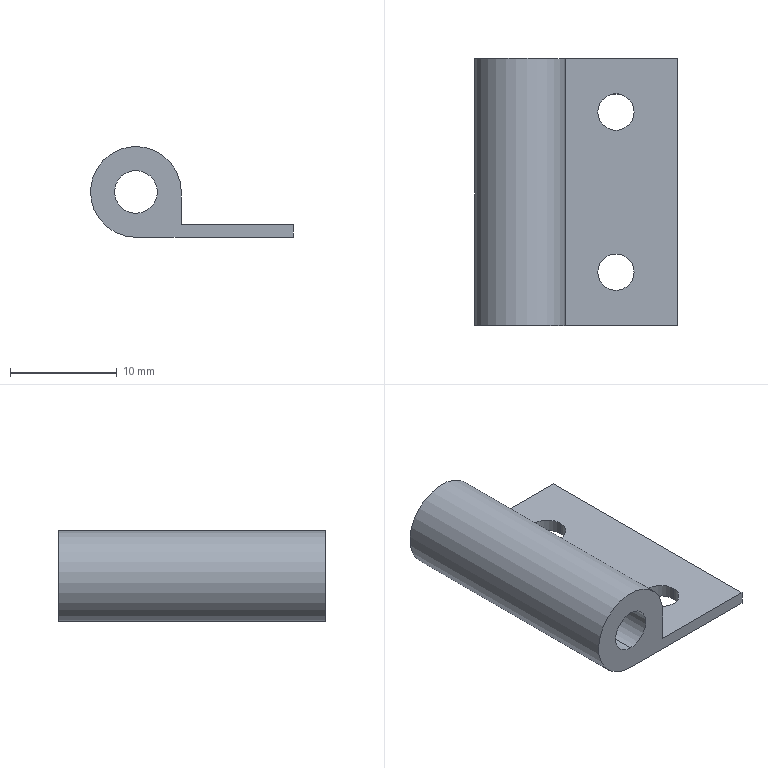Part | STEP file | Hinge CL237Z3H001-02 | 1 solid | 13 faces | box 19 x 25 x 8.5 mm | volume 1495 mm3 | cylinder 7 | plane 6 | commonest cylinder face diameters 3.4 x4 4 x2 8.5 x1
STEP:
#1=CARTESIAN_POINT('',(0.,0.,0.));
#2=DIRECTION('',(0.,0.,1.));
#3=DIRECTION('',(1.,0.,0.));
#4=AXIS2_PLACEMENT_3D('',#1,#2,#3);
#5=CARTESIAN_POINT('',(10.7,7.5,-4.25));
#6=VERTEX_POINT('',#5);
#7=CARTESIAN_POINT('',(10.7,7.5,-3.05));
#8=VERTEX_POINT('',#7);
#9=CARTESIAN_POINT('',(10.7,7.5,-3.05));
#10=DIRECTION('',(0.,0.,1.));
#11=VECTOR('',#10,1.);
#12=LINE('',#9,#11);
#13=CARTESIAN_POINT('',(9.,7.5,-3.05));
#14=DIRECTION('',(0.,0.,1.));
#15=DIRECTION('',(1.,0.,0.));
#16=AXIS2_PLACEMENT_3D('',#13,#14,#15);
#17=CYLINDRICAL_SURFACE('',#16,1.7);
#18=CARTESIAN_POINT('',(6.283,0.));
#19=DIRECTION('',(0.,1.));
#20=VECTOR('',#19,1.);
#21=LINE('',#18,#20);
#22=(GEOMETRIC_REPRESENTATION_CONTEXT(2)PARAMETRIC_REPRESENTATION_CONTEXT()REPRESENTATION_CONTEXT('',''));
#23=DEFINITIONAL_REPRESENTATION('',(#21),#22);
#24=PCURVE('',#17,#23);
#25=CARTESIAN_POINT('',(9.,7.5,-3.05));
#26=DIRECTION('',(0.,0.,1.));
#27=DIRECTION('',(1.,0.,0.));
#28=AXIS2_PLACEMENT_3D('',#25,#26,#27);
#29=CYLINDRICAL_SURFACE('',#28,1.7);
#30=CARTESIAN_POINT('',(0.,0.));
#31=DIRECTION('',(0.,1.));
#32=VECTOR('',#31,1.);
#33=LINE('',#30,#32);
#34=(GEOMETRIC_REPRESENTATION_CONTEXT(2)PARAMETRIC_REPRESENTATION_CONTEXT()REPRESENTATION_CONTEXT('',''));
#35=DEFINITIONAL_REPRESENTATION('',(#33),#34);
#36=PCURVE('',#29,#35);
#37=SURFACE_CURVE('',#12,(#24,#36),.PCURVE_S1.);
#38=EDGE_CURVE('',#6,#8,#37,.T.);
#39=ORIENTED_EDGE('',*,*,#38,.T.);
#40=CARTESIAN_POINT('',(7.3,7.5,-3.05));
#41=VERTEX_POINT('',#40);
#42=CARTESIAN_POINT('',(9.,7.5,-3.05));
#43=DIRECTION('',(0.,0.,1.));
#44=DIRECTION('',(1.,0.,0.));
#45=AXIS2_PLACEMENT_3D('',#42,#43,#44);
#46=CIRCLE('',#45,1.7);
#47=CARTESIAN_POINT('',(0.,0.));
#48=DIRECTION('',(1.,0.));
#49=VECTOR('',#48,1.);
#50=LINE('',#47,#49);
#51=(GEOMETRIC_REPRESENTATION_CONTEXT(2)PARAMETRIC_REPRESENTATION_CONTEXT()REPRESENTATION_CONTEXT('',''));
#52=DEFINITIONAL_REPRESENTATION('',(#50),#51);
#53=PCURVE('',#17,#52);
#54=CARTESIAN_POINT('',(14.75,12.5,-3.05));
#55=DIRECTION('',(0.,0.,-1.));
#56=DIRECTION('',(-1.,0.,0.));
#57=AXIS2_PLACEMENT_3D('',#54,#55,#56);
#58=PLANE('',#57);
#59=CARTESIAN_POINT('',(4.05,-5.));
#60=CARTESIAN_POINT('',(4.05,-2.056));
#61=CARTESIAN_POINT('',(6.6,-3.528));
#62=CARTESIAN_POINT('',(9.15,-5.));
#63=CARTESIAN_POINT('',(6.6,-6.472));
#64=CARTESIAN_POINT('',(4.05,-7.944));
#65=CARTESIAN_POINT('',(4.05,-5.));
#66=(BOUNDED_CURVE()B_SPLINE_CURVE(2,(#59,#60,#61,#62,#63,#64,#65),.UNSPECIFIED.,.T.,.F.)B_SPLINE_CURVE_WITH_KNOTS((1,2,2,2,2,1),(-2.094,0.,2.094,4.189,6.283,8.378),.UNSPECIFIED.)CURVE()GEOMETRIC_REPRESENTATION_ITEM()RATIONAL_B_SPLINE_CURVE((1.,0.5,1.,0.5,1.,0.5,1.))REPRESENTATION_ITEM(''));
#67=(GEOMETRIC_REPRESENTATION_CONTEXT(2)PARAMETRIC_REPRESENTATION_CONTEXT()REPRESENTATION_CONTEXT('',''));
#68=DEFINITIONAL_REPRESENTATION('',(#66),#67);
#69=PCURVE('',#58,#68);
#70=SURFACE_CURVE('',#46,(#53,#69),.PCURVE_S1.);
#71=EDGE_CURVE('',#41,#8,#70,.T.);
#72=ORIENTED_EDGE('',*,*,#71,.F.);
#73=CARTESIAN_POINT('',(7.3,7.5,-4.25));
#74=VERTEX_POINT('',#73);
#75=CARTESIAN_POINT('',(7.3,7.5,-3.05));
#76=DIRECTION('',(0.,0.,1.));
#77=VECTOR('',#76,1.);
#78=LINE('',#75,#77);
#79=CARTESIAN_POINT('',(3.142,0.));
#80=DIRECTION('',(0.,1.));
#81=VECTOR('',#80,1.);
#82=LINE('',#79,#81);
#83=(GEOMETRIC_REPRESENTATION_CONTEXT(2)PARAMETRIC_REPRESENTATION_CONTEXT()REPRESENTATION_CONTEXT('',''));
#84=DEFINITIONAL_REPRESENTATION('',(#82),#83);
#85=PCURVE('',#17,#84);
#86=CARTESIAN_POINT('',(3.142,0.));
#87=DIRECTION('',(0.,1.));
#88=VECTOR('',#87,1.);
#89=LINE('',#86,#88);
#90=(GEOMETRIC_REPRESENTATION_CONTEXT(2)PARAMETRIC_REPRESENTATION_CONTEXT()REPRESENTATION_CONTEXT('',''));
#91=DEFINITIONAL_REPRESENTATION('',(#89),#90);
#92=PCURVE('',#29,#91);
#93=SURFACE_CURVE('',#78,(#85,#92),.PCURVE_S1.);
#94=EDGE_CURVE('',#74,#41,#93,.T.);
#95=ORIENTED_EDGE('',*,*,#94,.F.);
#96=CARTESIAN_POINT('',(9.,7.5,-4.25));
#97=DIRECTION('',(0.,0.,1.));
#98=DIRECTION('',(1.,0.,0.));
#99=AXIS2_PLACEMENT_3D('',#96,#97,#98);
#100=CIRCLE('',#99,1.7);
#101=CARTESIAN_POINT('',(0.,-1.2));
#102=DIRECTION('',(1.,0.));
#103=VECTOR('',#102,1.);
#104=LINE('',#101,#103);
#105=(GEOMETRIC_REPRESENTATION_CONTEXT(2)PARAMETRIC_REPRESENTATION_CONTEXT()REPRESENTATION_CONTEXT('',''));
#106=DEFINITIONAL_REPRESENTATION('',(#104),#105);
#107=PCURVE('',#17,#106);
#108=CARTESIAN_POINT('',(0.,12.5,-4.25));
#109=DIRECTION('',(0.,0.,1.));
#110=DIRECTION('',(1.,0.,0.));
#111=AXIS2_PLACEMENT_3D('',#108,#109,#110);
#112=PLANE('',#111);
#113=CARTESIAN_POINT('',(9.,-5.));
#114=DIRECTION('',(1.,0.));
#115=AXIS2_PLACEMENT_2D('',#113,#114);
#116=CIRCLE('',#115,1.7);
#117=(GEOMETRIC_REPRESENTATION_CONTEXT(2)PARAMETRIC_REPRESENTATION_CONTEXT()REPRESENTATION_CONTEXT('',''));
#118=DEFINITIONAL_REPRESENTATION('',(#116),#117);
#119=PCURVE('',#112,#118);
#120=SURFACE_CURVE('',#100,(#107,#119),.PCURVE_S1.);
#121=EDGE_CURVE('',#74,#6,#120,.T.);
#122=ORIENTED_EDGE('',*,*,#121,.T.);
#123=EDGE_LOOP('',(#39,#72,#95,#122));
#124=FACE_BOUND('',#123,.F.);
#125=ADVANCED_FACE('',(#124),#17,.F.);
#126=CARTESIAN_POINT('',(10.7,-7.5,-4.25));
#127=VERTEX_POINT('',#126);
#128=CARTESIAN_POINT('',(10.7,-7.5,-3.05));
#129=VERTEX_POINT('',#128);
#130=CARTESIAN_POINT('',(10.7,-7.5,-3.05));
#131=DIRECTION('',(0.,0.,1.));
#132=VECTOR('',#131,1.);
#133=LINE('',#130,#132);
#134=CARTESIAN_POINT('',(9.,-7.5,-3.05));
#135=DIRECTION('',(0.,0.,1.));
#136=DIRECTION('',(1.,0.,0.));
#137=AXIS2_PLACEMENT_3D('',#134,#135,#136);
#138=CYLINDRICAL_SURFACE('',#137,1.7);
#139=CARTESIAN_POINT('',(6.283,0.));
#140=DIRECTION('',(0.,1.));
#141=VECTOR('',#140,1.);
#142=LINE('',#139,#141);
#143=(GEOMETRIC_REPRESENTATION_CONTEXT(2)PARAMETRIC_REPRESENTATION_CONTEXT()REPRESENTATION_CONTEXT('',''));
#144=DEFINITIONAL_REPRESENTATION('',(#142),#143);
#145=PCURVE('',#138,#144);
#146=CARTESIAN_POINT('',(9.,-7.5,-3.05));
#147=DIRECTION('',(0.,0.,1.));
#148=DIRECTION('',(1.,0.,0.));
#149=AXIS2_PLACEMENT_3D('',#146,#147,#148);
#150=CYLINDRICAL_SURFACE('',#149,1.7);
#151=CARTESIAN_POINT('',(0.,0.));
#152=DIRECTION('',(0.,1.));
#153=VECTOR('',#152,1.);
#154=LINE('',#151,#153);
#155=(GEOMETRIC_REPRESENTATION_CONTEXT(2)PARAMETRIC_REPRESENTATION_CONTEXT()REPRESENTATION_CONTEXT('',''));
#156=DEFINITIONAL_REPRESENTATION('',(#154),#155);
#157=PCURVE('',#150,#156);
#158=SURFACE_CURVE('',#133,(#145,#157),.PCURVE_S1.);
#159=EDGE_CURVE('',#127,#129,#158,.T.);
#160=ORIENTED_EDGE('',*,*,#159,.T.);
#161=CARTESIAN_POINT('',(7.3,-7.5,-3.05));
#162=VERTEX_POINT('',#161);
#163=CARTESIAN_POINT('',(9.,-7.5,-3.05));
#164=DIRECTION('',(0.,0.,1.));
#165=DIRECTION('',(1.,0.,0.));
#166=AXIS2_PLACEMENT_3D('',#163,#164,#165);
#167=CIRCLE('',#166,1.7);
#168=CARTESIAN_POINT('',(0.,0.));
#169=DIRECTION('',(1.,0.));
#170=VECTOR('',#169,1.);
#171=LINE('',#168,#170);
#172=(GEOMETRIC_REPRESENTATION_CONTEXT(2)PARAMETRIC_REPRESENTATION_CONTEXT()REPRESENTATION_CONTEXT('',''));
#173=DEFINITIONAL_REPRESENTATION('',(#171),#172);
#174=PCURVE('',#138,#173);
#175=CARTESIAN_POINT('',(4.05,-20.));
#176=CARTESIAN_POINT('',(4.05,-17.056));
#177=CARTESIAN_POINT('',(6.6,-18.528));
#178=CARTESIAN_POINT('',(9.15,-20.));
#179=CARTESIAN_POINT('',(6.6,-21.472));
#180=CARTESIAN_POINT('',(4.05,-22.944));
#181=CARTESIAN_POINT('',(4.05,-20.));
#182=(BOUNDED_CURVE()B_SPLINE_CURVE(2,(#175,#176,#177,#178,#179,#180,#181),.UNSPECIFIED.,.T.,.F.)B_SPLINE_CURVE_WITH_KNOTS((1,2,2,2,2,1),(-2.094,0.,2.094,4.189,6.283,8.378),.UNSPECIFIED.)CURVE()GEOMETRIC_REPRESENTATION_ITEM()RATIONAL_B_SPLINE_CURVE((1.,0.5,1.,0.5,1.,0.5,1.))REPRESENTATION_ITEM(''));
#183=(GEOMETRIC_REPRESENTATION_CONTEXT(2)PARAMETRIC_REPRESENTATION_CONTEXT()REPRESENTATION_CONTEXT('',''));
#184=DEFINITIONAL_REPRESENTATION('',(#182),#183);
#185=PCURVE('',#58,#184);
#186=SURFACE_CURVE('',#167,(#174,#185),.PCURVE_S1.);
#187=EDGE_CURVE('',#162,#129,#186,.T.);
#188=ORIENTED_EDGE('',*,*,#187,.F.);
#189=CARTESIAN_POINT('',(7.3,-7.5,-4.25));
#190=VERTEX_POINT('',#189);
#191=CARTESIAN_POINT('',(7.3,-7.5,-3.05));
#192=DIRECTION('',(0.,0.,1.));
#193=VECTOR('',#192,1.);
#194=LINE('',#191,#193);
#195=CARTESIAN_POINT('',(3.142,0.));
#196=DIRECTION('',(0.,1.));
#197=VECTOR('',#196,1.);
#198=LINE('',#195,#197);
#199=(GEOMETRIC_REPRESENTATION_CONTEXT(2)PARAMETRIC_REPRESENTATION_CONTEXT()REPRESENTATION_CONTEXT('',''));
#200=DEFINITIONAL_REPRESENTATION('',(#198),#199);
#201=PCURVE('',#138,#200);
#202=CARTESIAN_POINT('',(3.142,0.));
#203=DIRECTION('',(0.,1.));
#204=VECTOR('',#203,1.);
#205=LINE('',#202,#204);
#206=(GEOMETRIC_REPRESENTATION_CONTEXT(2)PARAMETRIC_REPRESENTATION_CONTEXT()REPRESENTATION_CONTEXT('',''));
#207=DEFINITIONAL_REPRESENTATION('',(#205),#206);
#208=PCURVE('',#150,#207);
#209=SURFACE_CURVE('',#194,(#201,#208),.PCURVE_S1.);
#210=EDGE_CURVE('',#190,#162,#209,.T.);
#211=ORIENTED_EDGE('',*,*,#210,.F.);
#212=CARTESIAN_POINT('',(9.,-7.5,-4.25));
#213=DIRECTION('',(0.,0.,1.));
#214=DIRECTION('',(1.,0.,0.));
#215=AXIS2_PLACEMENT_3D('',#212,#213,#214);
#216=CIRCLE('',#215,1.7);
#217=CARTESIAN_POINT('',(0.,-1.2));
#218=DIRECTION('',(1.,0.));
#219=VECTOR('',#218,1.);
#220=LINE('',#217,#219);
#221=(GEOMETRIC_REPRESENTATION_CONTEXT(2)PARAMETRIC_REPRESENTATION_CONTEXT()REPRESENTATION_CONTEXT('',''));
#222=DEFINITIONAL_REPRESENTATION('',(#220),#221);
#223=PCURVE('',#138,#222);
#224=CARTESIAN_POINT('',(9.,-20.));
#225=DIRECTION('',(1.,0.));
#226=AXIS2_PLACEMENT_2D('',#224,#225);
#227=CIRCLE('',#226,1.7);
#228=(GEOMETRIC_REPRESENTATION_CONTEXT(2)PARAMETRIC_REPRESENTATION_CONTEXT()REPRESENTATION_CONTEXT('',''));
#229=DEFINITIONAL_REPRESENTATION('',(#227),#228);
#230=PCURVE('',#112,#229);
#231=SURFACE_CURVE('',#216,(#223,#230),.PCURVE_S1.);
#232=EDGE_CURVE('',#190,#127,#231,.T.);
#233=ORIENTED_EDGE('',*,*,#232,.T.);
#234=EDGE_LOOP('',(#160,#188,#211,#233));
#235=FACE_BOUND('',#234,.F.);
#236=ADVANCED_FACE('',(#235),#138,.F.);
#237=CARTESIAN_POINT('',(0.,12.5,-2.));
#238=VERTEX_POINT('',#237);
#239=CARTESIAN_POINT('',(0.,-12.5,-2.));
#240=VERTEX_POINT('',#239);
#241=CARTESIAN_POINT('',(0.,12.5,-2.));
#242=DIRECTION('',(0.,-1.,0.));
#243=VECTOR('',#242,1.);
#244=LINE('',#241,#243);
#245=CARTESIAN_POINT('',(0.,12.5,0.));
#246=DIRECTION('',(0.,-1.,0.));
#247=DIRECTION('',(0.,0.,-1.));
#248=AXIS2_PLACEMENT_3D('',#245,#246,#247);
#249=CYLINDRICAL_SURFACE('',#248,2.);
#250=CARTESIAN_POINT('',(6.283,0.));
#251=DIRECTION('',(0.,1.));
#252=VECTOR('',#251,1.);
#253=LINE('',#250,#252);
#254=(GEOMETRIC_REPRESENTATION_CONTEXT(2)PARAMETRIC_REPRESENTATION_CONTEXT()REPRESENTATION_CONTEXT('',''));
#255=DEFINITIONAL_REPRESENTATION('',(#253),#254);
#256=PCURVE('',#249,#255);
#257=CARTESIAN_POINT('',(0.,12.5,0.));
#258=DIRECTION('',(0.,-1.,0.));
#259=DIRECTION('',(0.,0.,-1.));
#260=AXIS2_PLACEMENT_3D('',#257,#258,#259);
#261=CYLINDRICAL_SURFACE('',#260,2.);
#262=CARTESIAN_POINT('',(0.,0.));
#263=DIRECTION('',(0.,1.));
#264=VECTOR('',#263,1.);
#265=LINE('',#262,#264);
#266=(GEOMETRIC_REPRESENTATION_CONTEXT(2)PARAMETRIC_REPRESENTATION_CONTEXT()REPRESENTATION_CONTEXT('',''));
#267=DEFINITIONAL_REPRESENTATION('',(#265),#266);
#268=PCURVE('',#261,#267);
#269=SURFACE_CURVE('',#244,(#256,#268),.PCURVE_S1.);
#270=EDGE_CURVE('',#238,#240,#269,.T.);
#271=ORIENTED_EDGE('',*,*,#270,.T.);
#272=CARTESIAN_POINT('',(0.,-12.5,2.));
#273=VERTEX_POINT('',#272);
#274=CARTESIAN_POINT('',(0.,-12.5,0.));
#275=DIRECTION('',(0.,1.,0.));
#276=DIRECTION('',(0.,0.,1.));
#277=AXIS2_PLACEMENT_3D('',#274,#275,#276);
#278=CIRCLE('',#277,2.);
#279=CARTESIAN_POINT('',(9.425,25.));
#280=DIRECTION('',(-1.,0.));
#281=VECTOR('',#280,1.);
#282=LINE('',#279,#281);
#283=(GEOMETRIC_REPRESENTATION_CONTEXT(2)PARAMETRIC_REPRESENTATION_CONTEXT()REPRESENTATION_CONTEXT('',''));
#284=DEFINITIONAL_REPRESENTATION('',(#282),#283);
#285=PCURVE('',#249,#284);
#286=CARTESIAN_POINT('',(0.,-12.5,0.));
#287=DIRECTION('',(0.,1.,0.));
#288=DIRECTION('',(0.,0.,1.));
#289=AXIS2_PLACEMENT_3D('',#286,#287,#288);
#290=PLANE('',#289);
#291=CARTESIAN_POINT('',(0.,0.));
#292=DIRECTION('',(1.,0.));
#293=AXIS2_PLACEMENT_2D('',#291,#292);
#294=CIRCLE('',#293,2.);
#295=(GEOMETRIC_REPRESENTATION_CONTEXT(2)PARAMETRIC_REPRESENTATION_CONTEXT()REPRESENTATION_CONTEXT('',''));
#296=DEFINITIONAL_REPRESENTATION('',(#294),#295);
#297=PCURVE('',#290,#296);
#298=SURFACE_CURVE('',#278,(#285,#297),.PCURVE_S1.);
#299=EDGE_CURVE('',#240,#273,#298,.T.);
#300=ORIENTED_EDGE('',*,*,#299,.T.);
#301=CARTESIAN_POINT('',(0.,12.5,2.));
#302=VERTEX_POINT('',#301);
#303=CARTESIAN_POINT('',(0.,12.5,2.));
#304=DIRECTION('',(0.,-1.,0.));
#305=VECTOR('',#304,1.);
#306=LINE('',#303,#305);
#307=CARTESIAN_POINT('',(3.142,0.));
#308=DIRECTION('',(0.,1.));
#309=VECTOR('',#308,1.);
#310=LINE('',#307,#309);
#311=(GEOMETRIC_REPRESENTATION_CONTEXT(2)PARAMETRIC_REPRESENTATION_CONTEXT()REPRESENTATION_CONTEXT('',''));
#312=DEFINITIONAL_REPRESENTATION('',(#310),#311);
#313=PCURVE('',#249,#312);
#314=CARTESIAN_POINT('',(3.142,0.));
#315=DIRECTION('',(0.,1.));
#316=VECTOR('',#315,1.);
#317=LINE('',#314,#316);
#318=(GEOMETRIC_REPRESENTATION_CONTEXT(2)PARAMETRIC_REPRESENTATION_CONTEXT()REPRESENTATION_CONTEXT('',''));
#319=DEFINITIONAL_REPRESENTATION('',(#317),#318);
#320=PCURVE('',#261,#319);
#321=SURFACE_CURVE('',#306,(#313,#320),.PCURVE_S1.);
#322=EDGE_CURVE('',#302,#273,#321,.T.);
#323=ORIENTED_EDGE('',*,*,#322,.F.);
#324=CARTESIAN_POINT('',(0.,12.5,0.));
#325=DIRECTION('',(0.,1.,0.));
#326=DIRECTION('',(0.,0.,1.));
#327=AXIS2_PLACEMENT_3D('',#324,#325,#326);
#328=CIRCLE('',#327,2.);
#329=CARTESIAN_POINT('',(9.425,0.));
#330=DIRECTION('',(-1.,0.));
#331=VECTOR('',#330,1.);
#332=LINE('',#329,#331);
#333=(GEOMETRIC_REPRESENTATION_CONTEXT(2)PARAMETRIC_REPRESENTATION_CONTEXT()REPRESENTATION_CONTEXT('',''));
#334=DEFINITIONAL_REPRESENTATION('',(#332),#333);
#335=PCURVE('',#249,#334);
#336=CARTESIAN_POINT('',(0.,12.5,0.));
#337=DIRECTION('',(0.,1.,0.));
#338=DIRECTION('',(0.,0.,1.));
#339=AXIS2_PLACEMENT_3D('',#336,#337,#338);
#340=PLANE('',#339);
#341=CARTESIAN_POINT('',(0.,0.));
#342=DIRECTION('',(1.,0.));
#343=AXIS2_PLACEMENT_2D('',#341,#342);
#344=CIRCLE('',#343,2.);
#345=(GEOMETRIC_REPRESENTATION_CONTEXT(2)PARAMETRIC_REPRESENTATION_CONTEXT()REPRESENTATION_CONTEXT('',''));
#346=DEFINITIONAL_REPRESENTATION('',(#344),#345);
#347=PCURVE('',#340,#346);
#348=SURFACE_CURVE('',#328,(#335,#347),.PCURVE_S1.);
#349=EDGE_CURVE('',#238,#302,#348,.T.);
#350=ORIENTED_EDGE('',*,*,#349,.F.);
#351=EDGE_LOOP('',(#271,#300,#323,#350));
#352=FACE_BOUND('',#351,.F.);
#353=ADVANCED_FACE('',(#352),#249,.F.);
#354=CARTESIAN_POINT('',(0.,12.5,-4.25));
#355=VERTEX_POINT('',#354);
#356=CARTESIAN_POINT('',(4.25,12.5,0.));
#357=VERTEX_POINT('',#356);
#358=CARTESIAN_POINT('',(0.,12.5,0.));
#359=DIRECTION('',(0.,1.,0.));
#360=DIRECTION('',(0.,0.,1.));
#361=AXIS2_PLACEMENT_3D('',#358,#359,#360);
#362=CIRCLE('',#361,4.25);
#363=CARTESIAN_POINT('',(0.,0.));
#364=DIRECTION('',(1.,0.));
#365=AXIS2_PLACEMENT_2D('',#363,#364);
#366=CIRCLE('',#365,4.25);
#367=(GEOMETRIC_REPRESENTATION_CONTEXT(2)PARAMETRIC_REPRESENTATION_CONTEXT()REPRESENTATION_CONTEXT('',''));
#368=DEFINITIONAL_REPRESENTATION('',(#366),#367);
#369=PCURVE('',#340,#368);
#370=CARTESIAN_POINT('',(0.,12.5,0.));
#371=DIRECTION('',(0.,-1.,0.));
#372=DIRECTION('',(0.,0.,-1.));
#373=AXIS2_PLACEMENT_3D('',#370,#371,#372);
#374=CYLINDRICAL_SURFACE('',#373,4.25);
#375=CARTESIAN_POINT('',(9.425,0.));
#376=DIRECTION('',(-1.,0.));
#377=VECTOR('',#376,1.);
#378=LINE('',#375,#377);
#379=(GEOMETRIC_REPRESENTATION_CONTEXT(2)PARAMETRIC_REPRESENTATION_CONTEXT()REPRESENTATION_CONTEXT('',''));
#380=DEFINITIONAL_REPRESENTATION('',(#378),#379);
#381=PCURVE('',#374,#380);
#382=SURFACE_CURVE('',#362,(#369,#381),.PCURVE_S1.);
#383=EDGE_CURVE('',#355,#357,#382,.T.);
#384=ORIENTED_EDGE('',*,*,#383,.T.);
#385=CARTESIAN_POINT('',(4.25,12.5,-3.05));
#386=VERTEX_POINT('',#385);
#387=CARTESIAN_POINT('',(4.25,12.5,-3.05));
#388=DIRECTION('',(0.,0.,-1.));
#389=VECTOR('',#388,1.);
#390=LINE('',#387,#389);
#391=CARTESIAN_POINT('',(-3.05,4.25));
#392=DIRECTION('',(-1.,0.));
#393=VECTOR('',#392,1.);
#394=LINE('',#391,#393);
#395=(GEOMETRIC_REPRESENTATION_CONTEXT(2)PARAMETRIC_REPRESENTATION_CONTEXT()REPRESENTATION_CONTEXT('',''));
#396=DEFINITIONAL_REPRESENTATION('',(#394),#395);
#397=PCURVE('',#340,#396);
#398=CARTESIAN_POINT('',(4.25,12.5,-3.05));
#399=DIRECTION('',(-1.,0.,0.));
#400=DIRECTION('',(0.,0.,1.));
#401=AXIS2_PLACEMENT_3D('',#398,#399,#400);
#402=PLANE('',#401);
#403=CARTESIAN_POINT('',(0.,0.));
#404=DIRECTION('',(-1.,0.));
#405=VECTOR('',#404,1.);
#406=LINE('',#403,#405);
#407=(GEOMETRIC_REPRESENTATION_CONTEXT(2)PARAMETRIC_REPRESENTATION_CONTEXT()REPRESENTATION_CONTEXT('',''));
#408=DEFINITIONAL_REPRESENTATION('',(#406),#407);
#409=PCURVE('',#402,#408);
#410=SURFACE_CURVE('',#390,(#397,#409),.PCURVE_S1.);
#411=EDGE_CURVE('',#357,#386,#410,.T.);
#412=ORIENTED_EDGE('',*,*,#411,.T.);
#413=CARTESIAN_POINT('',(14.75,12.5,-3.05));
#414=VERTEX_POINT('',#413);
#415=CARTESIAN_POINT('',(14.75,12.5,-3.05));
#416=DIRECTION('',(1.,0.,0.));
#417=VECTOR('',#416,1.);
#418=LINE('',#415,#417);
#419=CARTESIAN_POINT('',(-3.05,14.75));
#420=DIRECTION('',(0.,1.));
#421=VECTOR('',#420,1.);
#422=LINE('',#419,#421);
#423=(GEOMETRIC_REPRESENTATION_CONTEXT(2)PARAMETRIC_REPRESENTATION_CONTEXT()REPRESENTATION_CONTEXT('',''));
#424=DEFINITIONAL_REPRESENTATION('',(#422),#423);
#425=PCURVE('',#340,#424);
#426=CARTESIAN_POINT('',(0.,0.));
#427=DIRECTION('',(-1.,0.));
#428=VECTOR('',#427,1.);
#429=LINE('',#426,#428);
#430=(GEOMETRIC_REPRESENTATION_CONTEXT(2)PARAMETRIC_REPRESENTATION_CONTEXT()REPRESENTATION_CONTEXT('',''));
#431=DEFINITIONAL_REPRESENTATION('',(#429),#430);
#432=PCURVE('',#58,#431);
#433=SURFACE_CURVE('',#418,(#425,#432),.PCURVE_S1.);
#434=EDGE_CURVE('',#386,#414,#433,.T.);
#435=ORIENTED_EDGE('',*,*,#434,.T.);
#436=CARTESIAN_POINT('',(14.75,12.5,-4.25));
#437=VERTEX_POINT('',#436);
#438=CARTESIAN_POINT('',(14.75,12.5,-4.25));
#439=DIRECTION('',(0.,0.,-1.));
#440=VECTOR('',#439,1.);
#441=LINE('',#438,#440);
#442=CARTESIAN_POINT('',(-4.25,14.75));
#443=DIRECTION('',(-1.,0.));
#444=VECTOR('',#443,1.);
#445=LINE('',#442,#444);
#446=(GEOMETRIC_REPRESENTATION_CONTEXT(2)PARAMETRIC_REPRESENTATION_CONTEXT()REPRESENTATION_CONTEXT('',''));
#447=DEFINITIONAL_REPRESENTATION('',(#445),#446);
#448=PCURVE('',#340,#447);
#449=CARTESIAN_POINT('',(14.75,12.5,-4.25));
#450=DIRECTION('',(-1.,0.,0.));
#451=DIRECTION('',(0.,0.,1.));
#452=AXIS2_PLACEMENT_3D('',#449,#450,#451);
#453=PLANE('',#452);
#454=CARTESIAN_POINT('',(0.,0.));
#455=DIRECTION('',(-1.,0.));
#456=VECTOR('',#455,1.);
#457=LINE('',#454,#456);
#458=(GEOMETRIC_REPRESENTATION_CONTEXT(2)PARAMETRIC_REPRESENTATION_CONTEXT()REPRESENTATION_CONTEXT('',''));
#459=DEFINITIONAL_REPRESENTATION('',(#457),#458);
#460=PCURVE('',#453,#459);
#461=SURFACE_CURVE('',#441,(#448,#460),.PCURVE_S1.);
#462=EDGE_CURVE('',#414,#437,#461,.T.);
#463=ORIENTED_EDGE('',*,*,#462,.T.);
#464=CARTESIAN_POINT('',(0.,12.5,-4.25));
#465=DIRECTION('',(-1.,0.,0.));
#466=VECTOR('',#465,1.);
#467=LINE('',#464,#466);
#468=CARTESIAN_POINT('',(-4.25,0.));
#469=DIRECTION('',(0.,-1.));
#470=VECTOR('',#469,1.);
#471=LINE('',#468,#470);
#472=(GEOMETRIC_REPRESENTATION_CONTEXT(2)PARAMETRIC_REPRESENTATION_CONTEXT()REPRESENTATION_CONTEXT('',''));
#473=DEFINITIONAL_REPRESENTATION('',(#471),#472);
#474=PCURVE('',#340,#473);
#475=CARTESIAN_POINT('',(0.,0.));
#476=DIRECTION('',(-1.,0.));
#477=VECTOR('',#476,1.);
#478=LINE('',#475,#477);
#479=(GEOMETRIC_REPRESENTATION_CONTEXT(2)PARAMETRIC_REPRESENTATION_CONTEXT()REPRESENTATION_CONTEXT('',''));
#480=DEFINITIONAL_REPRESENTATION('',(#478),#479);
#481=PCURVE('',#112,#480);
#482=SURFACE_CURVE('',#467,(#474,#481),.PCURVE_S1.);
#483=EDGE_CURVE('',#437,#355,#482,.T.);
#484=ORIENTED_EDGE('',*,*,#483,.T.);
#485=EDGE_LOOP('',(#384,#412,#435,#463,#484));
#486=FACE_BOUND('',#485,.T.);
#487=ORIENTED_EDGE('',*,*,#349,.F.);
#488=CARTESIAN_POINT('',(0.,12.5,0.));
#489=DIRECTION('',(0.,1.,0.));
#490=DIRECTION('',(0.,0.,1.));
#491=AXIS2_PLACEMENT_3D('',#488,#489,#490);
#492=CIRCLE('',#491,2.);
#493=CARTESIAN_POINT('',(0.,0.));
#494=DIRECTION('',(1.,0.));
#495=AXIS2_PLACEMENT_2D('',#493,#494);
#496=CIRCLE('',#495,2.);
#497=(GEOMETRIC_REPRESENTATION_CONTEXT(2)PARAMETRIC_REPRESENTATION_CONTEXT()REPRESENTATION_CONTEXT('',''));
#498=DEFINITIONAL_REPRESENTATION('',(#496),#497);
#499=PCURVE('',#340,#498);
#500=CARTESIAN_POINT('',(3.142,0.));
#501=DIRECTION('',(-1.,0.));
#502=VECTOR('',#501,1.);
#503=LINE('',#500,#502);
#504=(GEOMETRIC_REPRESENTATION_CONTEXT(2)PARAMETRIC_REPRESENTATION_CONTEXT()REPRESENTATION_CONTEXT('',''));
#505=DEFINITIONAL_REPRESENTATION('',(#503),#504);
#506=PCURVE('',#261,#505);
#507=SURFACE_CURVE('',#492,(#499,#506),.PCURVE_S1.);
#508=EDGE_CURVE('',#302,#238,#507,.T.);
#509=ORIENTED_EDGE('',*,*,#508,.F.);
#510=EDGE_LOOP('',(#487,#509));
#511=FACE_BOUND('',#510,.T.);
#512=ADVANCED_FACE('',(#486,#511),#340,.T.);
#513=CARTESIAN_POINT('',(0.,-12.5,-4.25));
#514=VERTEX_POINT('',#513);
#515=CARTESIAN_POINT('',(4.25,-12.5,0.));
#516=VERTEX_POINT('',#515);
#517=CARTESIAN_POINT('',(0.,-12.5,0.));
#518=DIRECTION('',(0.,1.,0.));
#519=DIRECTION('',(0.,0.,1.));
#520=AXIS2_PLACEMENT_3D('',#517,#518,#519);
#521=CIRCLE('',#520,4.25);
#522=CARTESIAN_POINT('',(0.,0.));
#523=DIRECTION('',(1.,0.));
#524=AXIS2_PLACEMENT_2D('',#522,#523);
#525=CIRCLE('',#524,4.25);
#526=(GEOMETRIC_REPRESENTATION_CONTEXT(2)PARAMETRIC_REPRESENTATION_CONTEXT()REPRESENTATION_CONTEXT('',''));
#527=DEFINITIONAL_REPRESENTATION('',(#525),#526);
#528=PCURVE('',#290,#527);
#529=CARTESIAN_POINT('',(9.425,25.));
#530=DIRECTION('',(-1.,0.));
#531=VECTOR('',#530,1.);
#532=LINE('',#529,#531);
#533=(GEOMETRIC_REPRESENTATION_CONTEXT(2)PARAMETRIC_REPRESENTATION_CONTEXT()REPRESENTATION_CONTEXT('',''));
#534=DEFINITIONAL_REPRESENTATION('',(#532),#533);
#535=PCURVE('',#374,#534);
#536=SURFACE_CURVE('',#521,(#528,#535),.PCURVE_S1.);
#537=EDGE_CURVE('',#514,#516,#536,.T.);
#538=ORIENTED_EDGE('',*,*,#537,.F.);
#539=CARTESIAN_POINT('',(14.75,-12.5,-4.25));
#540=VERTEX_POINT('',#539);
#541=CARTESIAN_POINT('',(0.,-12.5,-4.25));
#542=DIRECTION('',(-1.,0.,0.));
#543=VECTOR('',#542,1.);
#544=LINE('',#541,#543);
#545=CARTESIAN_POINT('',(-4.25,0.));
#546=DIRECTION('',(0.,-1.));
#547=VECTOR('',#546,1.);
#548=LINE('',#545,#547);
#549=(GEOMETRIC_REPRESENTATION_CONTEXT(2)PARAMETRIC_REPRESENTATION_CONTEXT()REPRESENTATION_CONTEXT('',''));
#550=DEFINITIONAL_REPRESENTATION('',(#548),#549);
#551=PCURVE('',#290,#550);
#552=CARTESIAN_POINT('',(0.,-25.));
#553=DIRECTION('',(-1.,0.));
#554=VECTOR('',#553,1.);
#555=LINE('',#552,#554);
#556=(GEOMETRIC_REPRESENTATION_CONTEXT(2)PARAMETRIC_REPRESENTATION_CONTEXT()REPRESENTATION_CONTEXT('',''));
#557=DEFINITIONAL_REPRESENTATION('',(#555),#556);
#558=PCURVE('',#112,#557);
#559=SURFACE_CURVE('',#544,(#551,#558),.PCURVE_S1.);
#560=EDGE_CURVE('',#540,#514,#559,.T.);
#561=ORIENTED_EDGE('',*,*,#560,.F.);
#562=CARTESIAN_POINT('',(14.75,-12.5,-3.05));
#563=VERTEX_POINT('',#562);
#564=CARTESIAN_POINT('',(14.75,-12.5,-4.25));
#565=DIRECTION('',(0.,0.,-1.));
#566=VECTOR('',#565,1.);
#567=LINE('',#564,#566);
#568=CARTESIAN_POINT('',(-4.25,14.75));
#569=DIRECTION('',(-1.,0.));
#570=VECTOR('',#569,1.);
#571=LINE('',#568,#570);
#572=(GEOMETRIC_REPRESENTATION_CONTEXT(2)PARAMETRIC_REPRESENTATION_CONTEXT()REPRESENTATION_CONTEXT('',''));
#573=DEFINITIONAL_REPRESENTATION('',(#571),#572);
#574=PCURVE('',#290,#573);
#575=CARTESIAN_POINT('',(0.,-25.));
#576=DIRECTION('',(-1.,0.));
#577=VECTOR('',#576,1.);
#578=LINE('',#575,#577);
#579=(GEOMETRIC_REPRESENTATION_CONTEXT(2)PARAMETRIC_REPRESENTATION_CONTEXT()REPRESENTATION_CONTEXT('',''));
#580=DEFINITIONAL_REPRESENTATION('',(#578),#579);
#581=PCURVE('',#453,#580);
#582=SURFACE_CURVE('',#567,(#574,#581),.PCURVE_S1.);
#583=EDGE_CURVE('',#563,#540,#582,.T.);
#584=ORIENTED_EDGE('',*,*,#583,.F.);
#585=CARTESIAN_POINT('',(4.25,-12.5,-3.05));
#586=VERTEX_POINT('',#585);
#587=CARTESIAN_POINT('',(14.75,-12.5,-3.05));
#588=DIRECTION('',(1.,0.,0.));
#589=VECTOR('',#588,1.);
#590=LINE('',#587,#589);
#591=CARTESIAN_POINT('',(-3.05,14.75));
#592=DIRECTION('',(0.,1.));
#593=VECTOR('',#592,1.);
#594=LINE('',#591,#593);
#595=(GEOMETRIC_REPRESENTATION_CONTEXT(2)PARAMETRIC_REPRESENTATION_CONTEXT()REPRESENTATION_CONTEXT('',''));
#596=DEFINITIONAL_REPRESENTATION('',(#594),#595);
#597=PCURVE('',#290,#596);
#598=CARTESIAN_POINT('',(0.,-25.));
#599=DIRECTION('',(-1.,0.));
#600=VECTOR('',#599,1.);
#601=LINE('',#598,#600);
#602=(GEOMETRIC_REPRESENTATION_CONTEXT(2)PARAMETRIC_REPRESENTATION_CONTEXT()REPRESENTATION_CONTEXT('',''));
#603=DEFINITIONAL_REPRESENTATION('',(#601),#602);
#604=PCURVE('',#58,#603);
#605=SURFACE_CURVE('',#590,(#597,#604),.PCURVE_S1.);
#606=EDGE_CURVE('',#586,#563,#605,.T.);
#607=ORIENTED_EDGE('',*,*,#606,.F.);
#608=CARTESIAN_POINT('',(4.25,-12.5,-3.05));
#609=DIRECTION('',(0.,0.,-1.));
#610=VECTOR('',#609,1.);
#611=LINE('',#608,#610);
#612=CARTESIAN_POINT('',(-3.05,4.25));
#613=DIRECTION('',(-1.,0.));
#614=VECTOR('',#613,1.);
#615=LINE('',#612,#614);
#616=(GEOMETRIC_REPRESENTATION_CONTEXT(2)PARAMETRIC_REPRESENTATION_CONTEXT()REPRESENTATION_CONTEXT('',''));
#617=DEFINITIONAL_REPRESENTATION('',(#615),#616);
#618=PCURVE('',#290,#617);
#619=CARTESIAN_POINT('',(0.,-25.));
#620=DIRECTION('',(-1.,0.));
#621=VECTOR('',#620,1.);
#622=LINE('',#619,#621);
#623=(GEOMETRIC_REPRESENTATION_CONTEXT(2)PARAMETRIC_REPRESENTATION_CONTEXT()REPRESENTATION_CONTEXT('',''));
#624=DEFINITIONAL_REPRESENTATION('',(#622),#623);
#625=PCURVE('',#402,#624);
#626=SURFACE_CURVE('',#611,(#618,#625),.PCURVE_S1.);
#627=EDGE_CURVE('',#516,#586,#626,.T.);
#628=ORIENTED_EDGE('',*,*,#627,.F.);
#629=EDGE_LOOP('',(#538,#561,#584,#607,#628));
#630=FACE_BOUND('',#629,.T.);
#631=ORIENTED_EDGE('',*,*,#299,.T.);
#632=CARTESIAN_POINT('',(0.,-12.5,0.));
#633=DIRECTION('',(0.,1.,0.));
#634=DIRECTION('',(0.,0.,1.));
#635=AXIS2_PLACEMENT_3D('',#632,#633,#634);
#636=CIRCLE('',#635,2.);
#637=CARTESIAN_POINT('',(0.,0.));
#638=DIRECTION('',(1.,0.));
#639=AXIS2_PLACEMENT_2D('',#637,#638);
#640=CIRCLE('',#639,2.);
#641=(GEOMETRIC_REPRESENTATION_CONTEXT(2)PARAMETRIC_REPRESENTATION_CONTEXT()REPRESENTATION_CONTEXT('',''));
#642=DEFINITIONAL_REPRESENTATION('',(#640),#641);
#643=PCURVE('',#290,#642);
#644=CARTESIAN_POINT('',(3.142,25.));
#645=DIRECTION('',(-1.,0.));
#646=VECTOR('',#645,1.);
#647=LINE('',#644,#646);
#648=(GEOMETRIC_REPRESENTATION_CONTEXT(2)PARAMETRIC_REPRESENTATION_CONTEXT()REPRESENTATION_CONTEXT('',''));
#649=DEFINITIONAL_REPRESENTATION('',(#647),#648);
#650=PCURVE('',#261,#649);
#651=SURFACE_CURVE('',#636,(#643,#650),.PCURVE_S1.);
#652=EDGE_CURVE('',#273,#240,#651,.T.);
#653=ORIENTED_EDGE('',*,*,#652,.T.);
#654=EDGE_LOOP('',(#631,#653));
#655=FACE_BOUND('',#654,.T.);
#656=ADVANCED_FACE('',(#630,#655),#290,.F.);
#657=ORIENTED_EDGE('',*,*,#537,.T.);
#658=CARTESIAN_POINT('',(4.25,12.5,0.));
#659=DIRECTION('',(0.,-1.,0.));
#660=VECTOR('',#659,1.);
#661=LINE('',#658,#660);
#662=CARTESIAN_POINT('',(1.571,0.));
#663=DIRECTION('',(0.,1.));
#664=VECTOR('',#663,1.);
#665=LINE('',#662,#664);
#666=(GEOMETRIC_REPRESENTATION_CONTEXT(2)PARAMETRIC_REPRESENTATION_CONTEXT()REPRESENTATION_CONTEXT('',''));
#667=DEFINITIONAL_REPRESENTATION('',(#665),#666);
#668=PCURVE('',#374,#667);
#669=CARTESIAN_POINT('',(3.05,0.));
#670=DIRECTION('',(0.,-1.));
#671=VECTOR('',#670,1.);
#672=LINE('',#669,#671);
#673=(GEOMETRIC_REPRESENTATION_CONTEXT(2)PARAMETRIC_REPRESENTATION_CONTEXT()REPRESENTATION_CONTEXT('',''));
#674=DEFINITIONAL_REPRESENTATION('',(#672),#673);
#675=PCURVE('',#402,#674);
#676=SURFACE_CURVE('',#661,(#668,#675),.PCURVE_S1.);
#677=EDGE_CURVE('',#357,#516,#676,.T.);
#678=ORIENTED_EDGE('',*,*,#677,.F.);
#679=ORIENTED_EDGE('',*,*,#383,.F.);
#680=CARTESIAN_POINT('',(0.,12.5,-4.25));
#681=DIRECTION('',(0.,-1.,0.));
#682=VECTOR('',#681,1.);
#683=LINE('',#680,#682);
#684=CARTESIAN_POINT('',(6.283,0.));
#685=DIRECTION('',(0.,1.));
#686=VECTOR('',#685,1.);
#687=LINE('',#684,#686);
#688=(GEOMETRIC_REPRESENTATION_CONTEXT(2)PARAMETRIC_REPRESENTATION_CONTEXT()REPRESENTATION_CONTEXT('',''));
#689=DEFINITIONAL_REPRESENTATION('',(#687),#688);
#690=PCURVE('',#374,#689);
#691=CARTESIAN_POINT('',(0.,0.));
#692=DIRECTION('',(0.,-1.));
#693=VECTOR('',#692,1.);
#694=LINE('',#691,#693);
#695=(GEOMETRIC_REPRESENTATION_CONTEXT(2)PARAMETRIC_REPRESENTATION_CONTEXT()REPRESENTATION_CONTEXT('',''));
#696=DEFINITIONAL_REPRESENTATION('',(#694),#695);
#697=PCURVE('',#112,#696);
#698=SURFACE_CURVE('',#683,(#690,#697),.PCURVE_S1.);
#699=EDGE_CURVE('',#355,#514,#698,.T.);
#700=ORIENTED_EDGE('',*,*,#699,.T.);
#701=EDGE_LOOP('',(#657,#678,#679,#700));
#702=FACE_BOUND('',#701,.T.);
#703=ADVANCED_FACE('',(#702),#374,.T.);
#704=ORIENTED_EDGE('',*,*,#627,.T.);
#705=CARTESIAN_POINT('',(4.25,12.5,-3.05));
#706=DIRECTION('',(0.,-1.,0.));
#707=VECTOR('',#706,1.);
#708=LINE('',#705,#707);
#709=CARTESIAN_POINT('',(0.,0.));
#710=DIRECTION('',(0.,-1.));
#711=VECTOR('',#710,1.);
#712=LINE('',#709,#711);
#713=(GEOMETRIC_REPRESENTATION_CONTEXT(2)PARAMETRIC_REPRESENTATION_CONTEXT()REPRESENTATION_CONTEXT('',''));
#714=DEFINITIONAL_REPRESENTATION('',(#712),#713);
#715=PCURVE('',#402,#714);
#716=CARTESIAN_POINT('',(10.5,0.));
#717=DIRECTION('',(0.,-1.));
#718=VECTOR('',#717,1.);
#719=LINE('',#716,#718);
#720=(GEOMETRIC_REPRESENTATION_CONTEXT(2)PARAMETRIC_REPRESENTATION_CONTEXT()REPRESENTATION_CONTEXT('',''));
#721=DEFINITIONAL_REPRESENTATION('',(#719),#720);
#722=PCURVE('',#58,#721);
#723=SURFACE_CURVE('',#708,(#715,#722),.PCURVE_S1.);
#724=EDGE_CURVE('',#386,#586,#723,.T.);
#725=ORIENTED_EDGE('',*,*,#724,.F.);
#726=ORIENTED_EDGE('',*,*,#411,.F.);
#727=ORIENTED_EDGE('',*,*,#677,.T.);
#728=EDGE_LOOP('',(#704,#725,#726,#727));
#729=FACE_BOUND('',#728,.T.);
#730=ADVANCED_FACE('',(#729),#402,.F.);
#731=CARTESIAN_POINT('',(9.,7.5,-3.05));
#732=DIRECTION('',(0.,0.,1.));
#733=DIRECTION('',(1.,0.,0.));
#734=AXIS2_PLACEMENT_3D('',#731,#732,#733);
#735=CIRCLE('',#734,1.7);
#736=CARTESIAN_POINT('',(4.05,-5.));
#737=CARTESIAN_POINT('',(4.05,-2.056));
#738=CARTESIAN_POINT('',(6.6,-3.528));
#739=CARTESIAN_POINT('',(9.15,-5.));
#740=CARTESIAN_POINT('',(6.6,-6.472));
#741=CARTESIAN_POINT('',(4.05,-7.944));
#742=CARTESIAN_POINT('',(4.05,-5.));
#743=(BOUNDED_CURVE()B_SPLINE_CURVE(2,(#736,#737,#738,#739,#740,#741,#742),.UNSPECIFIED.,.T.,.F.)B_SPLINE_CURVE_WITH_KNOTS((1,2,2,2,2,1),(-2.094,0.,2.094,4.189,6.283,8.378),.UNSPECIFIED.)CURVE()GEOMETRIC_REPRESENTATION_ITEM()RATIONAL_B_SPLINE_CURVE((1.,0.5,1.,0.5,1.,0.5,1.))REPRESENTATION_ITEM(''));
#744=(GEOMETRIC_REPRESENTATION_CONTEXT(2)PARAMETRIC_REPRESENTATION_CONTEXT()REPRESENTATION_CONTEXT('',''));
#745=DEFINITIONAL_REPRESENTATION('',(#743),#744);
#746=PCURVE('',#58,#745);
#747=CARTESIAN_POINT('',(0.,0.));
#748=DIRECTION('',(1.,0.));
#749=VECTOR('',#748,1.);
#750=LINE('',#747,#749);
#751=(GEOMETRIC_REPRESENTATION_CONTEXT(2)PARAMETRIC_REPRESENTATION_CONTEXT()REPRESENTATION_CONTEXT('',''));
#752=DEFINITIONAL_REPRESENTATION('',(#750),#751);
#753=PCURVE('',#29,#752);
#754=SURFACE_CURVE('',#735,(#746,#753),.PCURVE_S1.);
#755=EDGE_CURVE('',#8,#41,#754,.T.);
#756=ORIENTED_EDGE('',*,*,#755,.F.);
#757=ORIENTED_EDGE('',*,*,#71,.F.);
#758=EDGE_LOOP('',(#756,#757));
#759=FACE_BOUND('',#758,.T.);
#760=CARTESIAN_POINT('',(9.,-7.5,-3.05));
#761=DIRECTION('',(0.,0.,1.));
#762=DIRECTION('',(1.,0.,0.));
#763=AXIS2_PLACEMENT_3D('',#760,#761,#762);
#764=CIRCLE('',#763,1.7);
#765=CARTESIAN_POINT('',(4.05,-20.));
#766=CARTESIAN_POINT('',(4.05,-17.056));
#767=CARTESIAN_POINT('',(6.6,-18.528));
#768=CARTESIAN_POINT('',(9.15,-20.));
#769=CARTESIAN_POINT('',(6.6,-21.472));
#770=CARTESIAN_POINT('',(4.05,-22.944));
#771=CARTESIAN_POINT('',(4.05,-20.));
#772=(BOUNDED_CURVE()B_SPLINE_CURVE(2,(#765,#766,#767,#768,#769,#770,#771),.UNSPECIFIED.,.T.,.F.)B_SPLINE_CURVE_WITH_KNOTS((1,2,2,2,2,1),(-2.094,0.,2.094,4.189,6.283,8.378),.UNSPECIFIED.)CURVE()GEOMETRIC_REPRESENTATION_ITEM()RATIONAL_B_SPLINE_CURVE((1.,0.5,1.,0.5,1.,0.5,1.))REPRESENTATION_ITEM(''));
#773=(GEOMETRIC_REPRESENTATION_CONTEXT(2)PARAMETRIC_REPRESENTATION_CONTEXT()REPRESENTATION_CONTEXT('',''));
#774=DEFINITIONAL_REPRESENTATION('',(#772),#773);
#775=PCURVE('',#58,#774);
#776=CARTESIAN_POINT('',(0.,0.));
#777=DIRECTION('',(1.,0.));
#778=VECTOR('',#777,1.);
#779=LINE('',#776,#778);
#780=(GEOMETRIC_REPRESENTATION_CONTEXT(2)PARAMETRIC_REPRESENTATION_CONTEXT()REPRESENTATION_CONTEXT('',''));
#781=DEFINITIONAL_REPRESENTATION('',(#779),#780);
#782=PCURVE('',#150,#781);
#783=SURFACE_CURVE('',#764,(#775,#782),.PCURVE_S1.);
#784=EDGE_CURVE('',#129,#162,#783,.T.);
#785=ORIENTED_EDGE('',*,*,#784,.F.);
#786=ORIENTED_EDGE('',*,*,#187,.F.);
#787=EDGE_LOOP('',(#785,#786));
#788=FACE_BOUND('',#787,.T.);
#789=ORIENTED_EDGE('',*,*,#606,.T.);
#790=CARTESIAN_POINT('',(14.75,12.5,-3.05));
#791=DIRECTION('',(0.,-1.,0.));
#792=VECTOR('',#791,1.);
#793=LINE('',#790,#792);
#794=CARTESIAN_POINT('',(0.,0.));
#795=DIRECTION('',(0.,-1.));
#796=VECTOR('',#795,1.);
#797=LINE('',#794,#796);
#798=(GEOMETRIC_REPRESENTATION_CONTEXT(2)PARAMETRIC_REPRESENTATION_CONTEXT()REPRESENTATION_CONTEXT('',''));
#799=DEFINITIONAL_REPRESENTATION('',(#797),#798);
#800=PCURVE('',#58,#799);
#801=CARTESIAN_POINT('',(1.2,0.));
#802=DIRECTION('',(0.,-1.));
#803=VECTOR('',#802,1.);
#804=LINE('',#801,#803);
#805=(GEOMETRIC_REPRESENTATION_CONTEXT(2)PARAMETRIC_REPRESENTATION_CONTEXT()REPRESENTATION_CONTEXT('',''));
#806=DEFINITIONAL_REPRESENTATION('',(#804),#805);
#807=PCURVE('',#453,#806);
#808=SURFACE_CURVE('',#793,(#800,#807),.PCURVE_S1.);
#809=EDGE_CURVE('',#414,#563,#808,.T.);
#810=ORIENTED_EDGE('',*,*,#809,.F.);
#811=ORIENTED_EDGE('',*,*,#434,.F.);
#812=ORIENTED_EDGE('',*,*,#724,.T.);
#813=EDGE_LOOP('',(#789,#810,#811,#812));
#814=FACE_BOUND('',#813,.T.);
#815=ADVANCED_FACE('',(#759,#788,#814),#58,.F.);
#816=ORIENTED_EDGE('',*,*,#583,.T.);
#817=CARTESIAN_POINT('',(14.75,12.5,-4.25));
#818=DIRECTION('',(0.,-1.,0.));
#819=VECTOR('',#818,1.);
#820=LINE('',#817,#819);
#821=CARTESIAN_POINT('',(0.,0.));
#822=DIRECTION('',(0.,-1.));
#823=VECTOR('',#822,1.);
#824=LINE('',#821,#823);
#825=(GEOMETRIC_REPRESENTATION_CONTEXT(2)PARAMETRIC_REPRESENTATION_CONTEXT()REPRESENTATION_CONTEXT('',''));
#826=DEFINITIONAL_REPRESENTATION('',(#824),#825);
#827=PCURVE('',#453,#826);
#828=CARTESIAN_POINT('',(14.75,0.));
#829=DIRECTION('',(0.,-1.));
#830=VECTOR('',#829,1.);
#831=LINE('',#828,#830);
#832=(GEOMETRIC_REPRESENTATION_CONTEXT(2)PARAMETRIC_REPRESENTATION_CONTEXT()REPRESENTATION_CONTEXT('',''));
#833=DEFINITIONAL_REPRESENTATION('',(#831),#832);
#834=PCURVE('',#112,#833);
#835=SURFACE_CURVE('',#820,(#827,#834),.PCURVE_S1.);
#836=EDGE_CURVE('',#437,#540,#835,.T.);
#837=ORIENTED_EDGE('',*,*,#836,.F.);
#838=ORIENTED_EDGE('',*,*,#462,.F.);
#839=ORIENTED_EDGE('',*,*,#809,.T.);
#840=EDGE_LOOP('',(#816,#837,#838,#839));
#841=FACE_BOUND('',#840,.T.);
#842=ADVANCED_FACE('',(#841),#453,.F.);
#843=CARTESIAN_POINT('',(9.,7.5,-4.25));
#844=DIRECTION('',(0.,0.,1.));
#845=DIRECTION('',(1.,0.,0.));
#846=AXIS2_PLACEMENT_3D('',#843,#844,#845);
#847=CIRCLE('',#846,1.7);
#848=CARTESIAN_POINT('',(9.,-5.));
#849=DIRECTION('',(1.,0.));
#850=AXIS2_PLACEMENT_2D('',#848,#849);
#851=CIRCLE('',#850,1.7);
#852=(GEOMETRIC_REPRESENTATION_CONTEXT(2)PARAMETRIC_REPRESENTATION_CONTEXT()REPRESENTATION_CONTEXT('',''));
#853=DEFINITIONAL_REPRESENTATION('',(#851),#852);
#854=PCURVE('',#112,#853);
#855=CARTESIAN_POINT('',(0.,-1.2));
#856=DIRECTION('',(1.,0.));
#857=VECTOR('',#856,1.);
#858=LINE('',#855,#857);
#859=(GEOMETRIC_REPRESENTATION_CONTEXT(2)PARAMETRIC_REPRESENTATION_CONTEXT()REPRESENTATION_CONTEXT('',''));
#860=DEFINITIONAL_REPRESENTATION('',(#858),#859);
#861=PCURVE('',#29,#860);
#862=SURFACE_CURVE('',#847,(#854,#861),.PCURVE_S1.);
#863=EDGE_CURVE('',#6,#74,#862,.T.);
#864=ORIENTED_EDGE('',*,*,#863,.T.);
#865=ORIENTED_EDGE('',*,*,#121,.T.);
#866=EDGE_LOOP('',(#864,#865));
#867=FACE_BOUND('',#866,.T.);
#868=CARTESIAN_POINT('',(9.,-7.5,-4.25));
#869=DIRECTION('',(0.,0.,1.));
#870=DIRECTION('',(1.,0.,0.));
#871=AXIS2_PLACEMENT_3D('',#868,#869,#870);
#872=CIRCLE('',#871,1.7);
#873=CARTESIAN_POINT('',(9.,-20.));
#874=DIRECTION('',(1.,0.));
#875=AXIS2_PLACEMENT_2D('',#873,#874);
#876=CIRCLE('',#875,1.7);
#877=(GEOMETRIC_REPRESENTATION_CONTEXT(2)PARAMETRIC_REPRESENTATION_CONTEXT()REPRESENTATION_CONTEXT('',''));
#878=DEFINITIONAL_REPRESENTATION('',(#876),#877);
#879=PCURVE('',#112,#878);
#880=CARTESIAN_POINT('',(0.,-1.2));
#881=DIRECTION('',(1.,0.));
#882=VECTOR('',#881,1.);
#883=LINE('',#880,#882);
#884=(GEOMETRIC_REPRESENTATION_CONTEXT(2)PARAMETRIC_REPRESENTATION_CONTEXT()REPRESENTATION_CONTEXT('',''));
#885=DEFINITIONAL_REPRESENTATION('',(#883),#884);
#886=PCURVE('',#150,#885);
#887=SURFACE_CURVE('',#872,(#879,#886),.PCURVE_S1.);
#888=EDGE_CURVE('',#127,#190,#887,.T.);
#889=ORIENTED_EDGE('',*,*,#888,.T.);
#890=ORIENTED_EDGE('',*,*,#232,.T.);
#891=EDGE_LOOP('',(#889,#890));
#892=FACE_BOUND('',#891,.T.);
#893=ORIENTED_EDGE('',*,*,#560,.T.);
#894=ORIENTED_EDGE('',*,*,#699,.F.);
#895=ORIENTED_EDGE('',*,*,#483,.F.);
#896=ORIENTED_EDGE('',*,*,#836,.T.);
#897=EDGE_LOOP('',(#893,#894,#895,#896));
#898=FACE_BOUND('',#897,.T.);
#899=ADVANCED_FACE('',(#867,#892,#898),#112,.F.);
#900=ORIENTED_EDGE('',*,*,#652,.T.);
#901=ORIENTED_EDGE('',*,*,#270,.F.);
#902=ORIENTED_EDGE('',*,*,#508,.F.);
#903=ORIENTED_EDGE('',*,*,#322,.T.);
#904=EDGE_LOOP('',(#900,#901,#902,#903));
#905=FACE_BOUND('',#904,.F.);
#906=ADVANCED_FACE('',(#905),#261,.F.);
#907=ORIENTED_EDGE('',*,*,#784,.F.);
#908=ORIENTED_EDGE('',*,*,#159,.F.);
#909=ORIENTED_EDGE('',*,*,#888,.T.);
#910=ORIENTED_EDGE('',*,*,#210,.T.);
#911=EDGE_LOOP('',(#907,#908,#909,#910));
#912=FACE_BOUND('',#911,.F.);
#913=ADVANCED_FACE('',(#912),#150,.F.);
#914=ORIENTED_EDGE('',*,*,#755,.F.);
#915=ORIENTED_EDGE('',*,*,#38,.F.);
#916=ORIENTED_EDGE('',*,*,#863,.T.);
#917=ORIENTED_EDGE('',*,*,#94,.T.);
#918=EDGE_LOOP('',(#914,#915,#916,#917));
#919=FACE_BOUND('',#918,.F.);
#920=ADVANCED_FACE('',(#919),#29,.F.);
#921=CLOSED_SHELL('',(#125,#236,#353,#512,#656,#703,#730,#815,#842,#899,#906,#913,#920));
#922=MANIFOLD_SOLID_BREP('',#921);
#923=(LENGTH_UNIT()NAMED_UNIT(*)SI_UNIT(.MILLI.,.METRE.));
#924=UNCERTAINTY_MEASURE_WITH_UNIT(LENGTH_MEASURE(0.0000001),#923,'','');
#925=(NAMED_UNIT(*)PLANE_ANGLE_UNIT()SI_UNIT($,.RADIAN.));
#926=(NAMED_UNIT(*)SI_UNIT($,.STERADIAN.)SOLID_ANGLE_UNIT());
#927=(GEOMETRIC_REPRESENTATION_CONTEXT(3)GLOBAL_UNCERTAINTY_ASSIGNED_CONTEXT((#924))GLOBAL_UNIT_ASSIGNED_CONTEXT((#923,#925,#926))REPRESENTATION_CONTEXT('',''));
#928=ADVANCED_BREP_SHAPE_REPRESENTATION('',(#4,#922),#927);